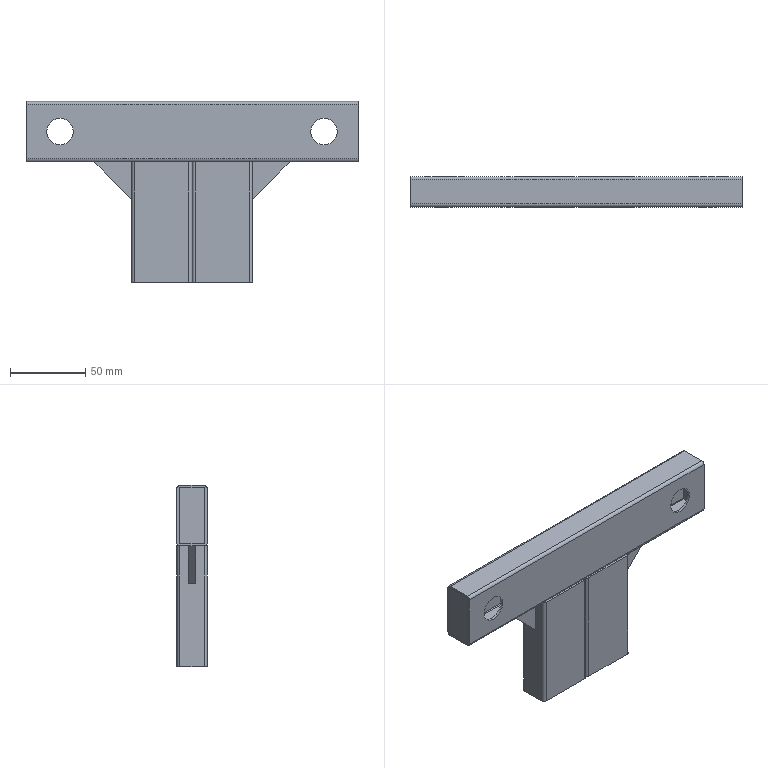Part | STEP file | 18-Top post_default<machined> | 9 solids | 112 faces | box 220 x 20 x 120 mm | volume 67083 mm3 | plane 64 | cylinder 48 | commonest cylinder face diameters 1 x28 4 x12 17.5 x4 26 x4